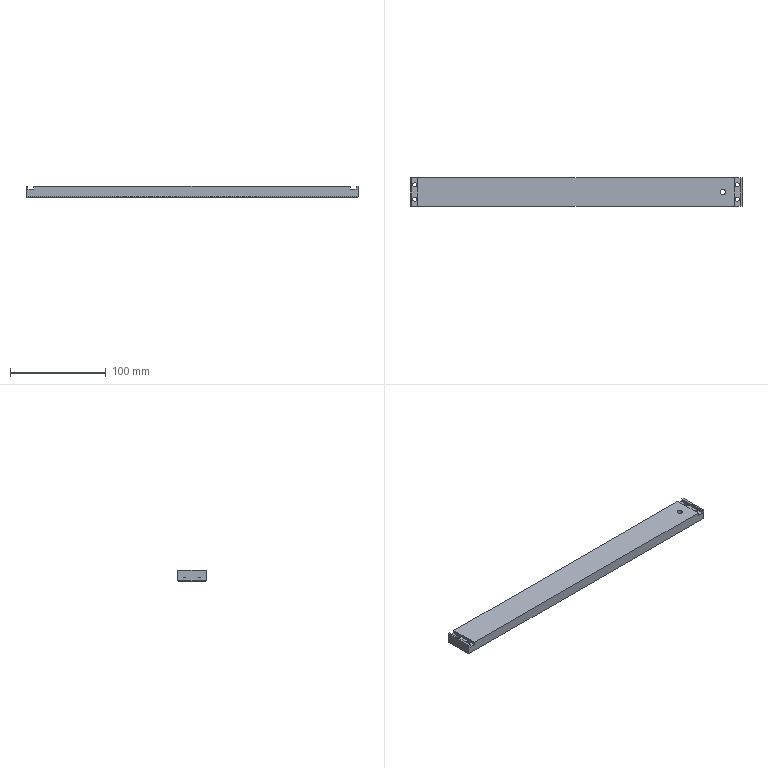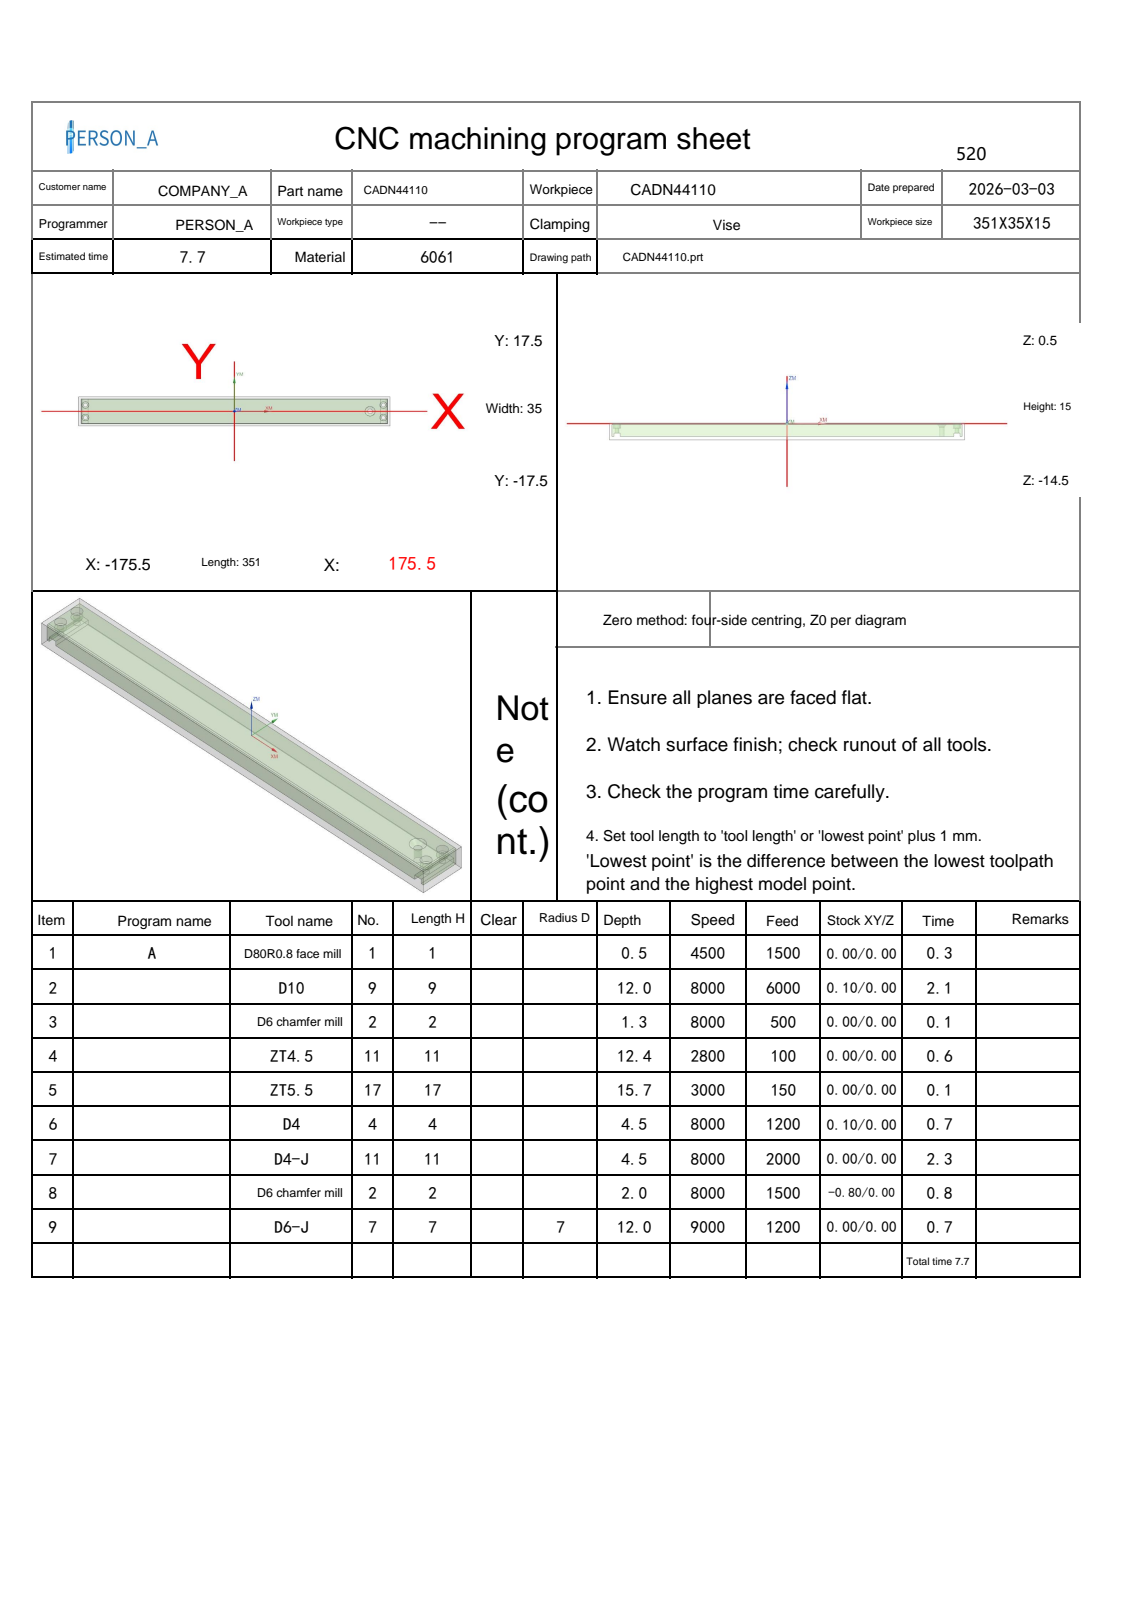NC program | NX | posted by the shop | part box 346 x 30 x 11.5 mm
Lines 1 to 336 of 28539:
%
O0001
(Machine time: 9.54 MIN)
(===Total Tool:7===)
(T1=D80R0.8 face mill D=80. R=0.8 D- H01 Z=0.    )
(T9=D10     D=10.  R=0.   D-  H09 Z=-11.5 )
(T2=D6 chamfer mill D=6. R=0. D- H02 Z=-1.5  )
(T11=ZT4.5  D=4.5  DR_a=118 D-  H11 Z=-11.85)
(T17=ZT5.5  D=5.5  DR_a=118 D-  H17 Z=-15.15)
(T4=D4      D=4.   R=0.   D-  H04 Z=-4.   )
(T7=D6-J    D=6.   R=0.   D7  H07 Z=-11.5 )
G80 G90 G17 G49 G40
G91 G28 Z0
M01
N1 T01 M06
(D80R0.8 face mill D=80. R=0.8 H=01 ce=0.00 di=0.00)
G00 G90 G54 X218. Y0.0 M03 S4500
G43 H01 Z30.
M08
Z2.
G01 Z0.0 F1500.
X213.
X-213.
X-218.
Z2.
G00 Z30.
G91 G28 Z0.0
M05
M09
G91 G28 Z0.0
M01
N2 T09 M06
(D10  D=10. R=0. H=09 ce=0.10 di=0.00)
G00 G90 G54 X0.0 Y20.1 M03 S8000
G43 H09 Z30.
M08
Z.5
G01 X173. Z.323 F6000.
G02 X178.1 Y15. Z.315 I0.0 J-5.1
G01 Y-15. Z.285
G02 X173. Y-20.1 Z.277 I-5.1 J0.0
G01 X-173. Z-.077
G02 X-178.1 Y-15. Z-.085 I0.0 J5.1
G01 Y15. Z-.115
G02 X-173. Y20.1 Z-.123 I5.1 J0.0
G01 X173. Z-.477
G02 X178.1 Y15. Z-.485 I0.0 J-5.1
G01 Y-15. Z-.515
G02 X173. Y-20.1 Z-.523 I-5.1 J0.0
G01 X-173. Z-.877
G02 X-178.1 Y-15. Z-.885 I0.0 J5.1
G01 Y15. Z-.915
G02 X-173. Y20.1 Z-.923 I5.1 J0.0
G01 X173. Z-1.277
G02 X178.1 Y15. Z-1.285 I0.0 J-5.1
G01 Y-15. Z-1.315
G02 X173. Y-20.1 Z-1.323 I-5.1 J0.0
G01 X-173. Z-1.677
G02 X-178.1 Y-15. Z-1.685 I0.0 J5.1
G01 Y15. Z-1.715
G02 X-173. Y20.1 Z-1.723 I5.1 J0.0
G01 X173. Z-2.077
G02 X178.1 Y15. Z-2.085 I0.0 J-5.1
G01 Y-15. Z-2.115
G02 X173. Y-20.1 Z-2.123 I-5.1 J0.0
G01 X-173. Z-2.477
G02 X-178.1 Y-15. Z-2.485 I0.0 J5.1
G01 Y15. Z-2.515
G02 X-173. Y20.1 Z-2.523 I5.1 J0.0
G01 X173. Z-2.877
G02 X178.1 Y15. Z-2.885 I0.0 J-5.1
G01 Y-15. Z-2.915
G02 X173. Y-20.1 Z-2.923 I-5.1 J0.0
G01 X-173. Z-3.277
G02 X-178.1 Y-15. Z-3.285 I0.0 J5.1
G01 Y15. Z-3.315
G02 X-173. Y20.1 Z-3.323 I5.1 J0.0
G01 X173. Z-3.677
G02 X178.1 Y15. Z-3.685 I0.0 J-5.1
G01 Y-15. Z-3.715
G02 X173. Y-20.1 Z-3.723 I-5.1 J0.0
G01 X-173. Z-4.077
G02 X-178.1 Y-15. Z-4.085 I0.0 J5.1
G01 Y15. Z-4.115
G02 X-173. Y20.1 Z-4.123 I5.1 J0.0
G01 X173. Z-4.477
G02 X178.1 Y15. Z-4.485 I0.0 J-5.1
G01 Y-15. Z-4.515
G02 X173. Y-20.1 Z-4.523 I-5.1 J0.0
G01 X-173. Z-4.877
G02 X-178.1 Y-15. Z-4.885 I0.0 J5.1
G01 Y15. Z-4.915
G02 X-173. Y20.1 Z-4.923 I5.1 J0.0
G01 X173. Z-5.277
G02 X178.1 Y15. Z-5.285 I0.0 J-5.1
G01 Y-15. Z-5.315
G02 X173. Y-20.1 Z-5.323 I-5.1 J0.0
G01 X-173. Z-5.677
G02 X-178.1 Y-15. Z-5.685 I0.0 J5.1
G01 Y15. Z-5.715
G02 X-173. Y20.1 Z-5.723 I5.1 J0.0
G01 X173. Z-6.077
G02 X178.1 Y15. Z-6.085 I0.0 J-5.1
G01 Y-15. Z-6.115
G02 X173. Y-20.1 Z-6.123 I-5.1 J0.0
G01 X-173. Z-6.477
G02 X-178.1 Y-15. Z-6.485 I0.0 J5.1
G01 Y15. Z-6.515
G02 X-173. Y20.1 Z-6.523 I5.1 J0.0
G01 X173. Z-6.877
G02 X178.1 Y15. Z-6.885 I0.0 J-5.1
G01 Y-15. Z-6.915
G02 X173. Y-20.1 Z-6.923 I-5.1 J0.0
G01 X-173. Z-7.277
G02 X-178.1 Y-15. Z-7.285 I0.0 J5.1
G01 Y15. Z-7.315
G02 X-173. Y20.1 Z-7.323 I5.1 J0.0
G01 X173. Z-7.677
G02 X178.1 Y15. Z-7.685 I0.0 J-5.1
G01 Y-15. Z-7.715
G02 X173. Y-20.1 Z-7.723 I-5.1 J0.0
G01 X-173. Z-8.077
G02 X-178.1 Y-15. Z-8.085 I0.0 J5.1
G01 Y15. Z-8.115
G02 X-173. Y20.1 Z-8.123 I5.1 J0.0
G01 X173. Z-8.477
G02 X178.1 Y15. Z-8.485 I0.0 J-5.1
G01 Y-15. Z-8.515
G02 X173. Y-20.1 Z-8.523 I-5.1 J0.0
G01 X-173. Z-8.877
G02 X-178.1 Y-15. Z-8.885 I0.0 J5.1
G01 Y15. Z-8.915
G02 X-173. Y20.1 Z-8.923 I5.1 J0.0
G01 X173. Z-9.277
G02 X178.1 Y15. Z-9.285 I0.0 J-5.1
G01 Y-15. Z-9.315
G02 X173. Y-20.1 Z-9.323 I-5.1 J0.0
G01 X-173. Z-9.677
G02 X-178.1 Y-15. Z-9.685 I0.0 J5.1
G01 Y15. Z-9.715
G02 X-173. Y20.1 Z-9.723 I5.1 J0.0
G01 X173. Z-10.077
G02 X178.1 Y15. Z-10.085 I0.0 J-5.1
G01 Y-15. Z-10.115
G02 X173. Y-20.1 Z-10.123 I-5.1 J0.0
G01 X-173. Z-10.477
G02 X-178.1 Y-15. Z-10.485 I0.0 J5.1
G01 Y15. Z-10.515
G02 X-173. Y20.1 Z-10.523 I5.1 J0.0
G01 X173. Z-10.877
G02 X178.1 Y15. Z-10.885 I0.0 J-5.1
G01 Y-15. Z-10.915
G02 X173. Y-20.1 Z-10.923 I-5.1 J0.0
G01 X-173. Z-11.277
G02 X-178.1 Y-15. Z-11.285 I0.0 J5.1
G01 Y15. Z-11.315
G02 X-173. Y20.1 Z-11.323 I5.1 J0.0
G01 X0.0 Z-11.5
X173.
G02 X178.1 Y15. I0.0 J-5.1
G01 Y-15.
G02 X173. Y-20.1 I-5.1 J0.0
G01 X-173.
G02 X-178.1 Y-15. I0.0 J5.1
G01 Y15.
G02 X-173. Y20.1 I5.1 J0.0
G01 X0.0
X.5
Z-10.5
G00 Z30.
G91 G28 Z0.0
M05
M09
G91 G28 Z0.0
M01
N3 T02 M06
(D6 chamfer mill D=6. R=0. H=02 ce=0.00 di=0.00)
G00 G90 G54 X168. Y7.5 M03 S8000
G43 H02 Z30.
M08
G98 G81 X168. Y7.5 Z-.8 R1. F500.
Y-7.5
X153. Y0.0
X-168. Y7.5
Y-7.5
G80
G00 Z30.
G91 G28 Z0.0
M05
M09
G91 G28 Z0.0
M01
N4 T11 M06
(ZT4.5 D=4.5 DR_a=118 H=11)
G00 G90 G54 X168. Y7.5 M03 S2800
G43 H11 Z30.
M08
G98 G83 X168. Y7.5 Z-11.852 R1. F100. Q2.
Y-7.5
X-168.
Y7.5
G80
G00 Z30.
G91 G28 Z0.0
M05
M09
G91 G28 Z0.0
M01
N5 T17 M06
(ZT5.5 D=5.5 DR_a=118 H=17)
G00 G90 G54 X153. Y0.0 M03 S3000
G43 H17 Z30.
M08
G98 G83 X153. Y0.0 Z-15.152 R1. F150. Q3.
G80
G00 Z30.
G91 G28 Z0.0
M05
M09
G91 G28 Z0.0
M01
N6 T04 M06
(D4  D=4. R=0. H=04 ce=0.10 di=0.00)
G00 G90 G54 X168. Y7.5 M03 S8000
G43 H04 Z30.
M08
Z.5
G03 X168.95 Y6.55 I.95 J0.0 F1200.
X169.9 Y7.5 I0.0 J.95
X169.9 Y7.5 Z.2 I-1.9 J0.0
X169.9 Y7.5 Z-.1 I-1.9 J0.0
X169.9 Y7.5 Z-.4 I-1.9 J0.0
X169.9 Y7.5 Z-.7 I-1.9 J0.0
X169.9 Y7.5 Z-1. I-1.9 J0.0
X169.9 Y7.5 Z-1.3 I-1.9 J0.0
X169.9 Y7.5 Z-1.6 I-1.9 J0.0
X169.9 Y7.5 Z-1.9 I-1.9 J0.0
X169.9 Y7.5 Z-2.2 I-1.9 J0.0
X169.9 Y7.5 Z-2.5 I-1.9 J0.0
X169.9 Y7.5 Z-2.8 I-1.9 J0.0
X169.9 Y7.5 Z-3.1 I-1.9 J0.0
X169.9 Y7.5 Z-3.4 I-1.9 J0.0
X169.9 Y7.5 Z-3.7 I-1.9 J0.0
X169.9 Y7.5 Z-4. I-1.9 J0.0
X168. Y9.4 I-1.9 J0.0
X166.1 Y7.5 I0.0 J-1.9
X168. Y5.6 I1.9 J0.0
X169.9 Y7.5 I0.0 J1.9
X168.95 Y8.45 I-.95 J0.0
X168. Y7.5 I0.0 J-.95
G00 Z30.
Y-7.5
Z.5
G03 X168.95 Y-8.45 I.95 J0.0
X169.9 Y-7.5 I0.0 J.95
X169.9 Y-7.5 Z.2 I-1.9 J0.0
X169.9 Y-7.5 Z-.1 I-1.9 J0.0
X169.9 Y-7.5 Z-.4 I-1.9 J0.0
X169.9 Y-7.5 Z-.7 I-1.9 J0.0
X169.9 Y-7.5 Z-1. I-1.9 J0.0
X169.9 Y-7.5 Z-1.3 I-1.9 J0.0
X169.9 Y-7.5 Z-1.6 I-1.9 J0.0
X169.9 Y-7.5 Z-1.9 I-1.9 J0.0
X169.9 Y-7.5 Z-2.2 I-1.9 J0.0
X169.9 Y-7.5 Z-2.5 I-1.9 J0.0
X169.9 Y-7.5 Z-2.8 I-1.9 J0.0
X169.9 Y-7.5 Z-3.1 I-1.9 J0.0
X169.9 Y-7.5 Z-3.4 I-1.9 J0.0
X169.9 Y-7.5 Z-3.7 I-1.9 J0.0
X169.9 Y-7.5 Z-4. I-1.9 J0.0
X168. Y-5.6 I-1.9 J0.0
X166.1 Y-7.5 I0.0 J-1.9
X168. Y-9.4 I1.9 J0.0
X169.9 Y-7.5 I0.0 J1.9
X168.95 Y-6.55 I-.95 J0.0
X168. Y-7.5 I0.0 J-.95
G00 Z30.
X-168.
Z.5
G03 X-167.05 Y-8.45 I.95 J0.0
X-166.1 Y-7.5 I0.0 J.95
X-166.1 Y-7.5 Z.2 I-1.9 J0.0
X-166.1 Y-7.5 Z-.1 I-1.9 J0.0
X-166.1 Y-7.5 Z-.4 I-1.9 J0.0
X-166.1 Y-7.5 Z-.7 I-1.9 J0.0
X-166.1 Y-7.5 Z-1. I-1.9 J0.0
X-166.1 Y-7.5 Z-1.3 I-1.9 J0.0
X-166.1 Y-7.5 Z-1.6 I-1.9 J0.0
X-166.1 Y-7.5 Z-1.9 I-1.9 J0.0
X-166.1 Y-7.5 Z-2.2 I-1.9 J0.0
X-166.1 Y-7.5 Z-2.5 I-1.9 J0.0
X-166.1 Y-7.5 Z-2.8 I-1.9 J0.0
X-166.1 Y-7.5 Z-3.1 I-1.9 J0.0
X-166.1 Y-7.5 Z-3.4 I-1.9 J0.0
X-166.1 Y-7.5 Z-3.7 I-1.9 J0.0
X-166.1 Y-7.5 Z-4. I-1.9 J0.0
X-168. Y-5.6 I-1.9 J0.0
X-169.9 Y-7.5 I0.0 J-1.9
X-168. Y-9.4 I1.9 J0.0
X-166.1 Y-7.5 I0.0 J1.9
X-167.05 Y-6.55 I-.95 J0.0
X-168. Y-7.5 I0.0 J-.95
G00 Z30.
Y7.5
Z.5
G03 X-167.05 Y6.55 I.95 J0.0
X-166.1 Y7.5 I0.0 J.95
X-166.1 Y7.5 Z.2 I-1.9 J0.0
X-166.1 Y7.5 Z-.1 I-1.9 J0.0
X-166.1 Y7.5 Z-.4 I-1.9 J0.0
X-166.1 Y7.5 Z-.7 I-1.9 J0.0
X-166.1 Y7.5 Z-1. I-1.9 J0.0
X-166.1 Y7.5 Z-1.3 I-1.9 J0.0
X-166.1 Y7.5 Z-1.6 I-1.9 J0.0
X-166.1 Y7.5 Z-1.9 I-1.9 J0.0
X-166.1 Y7.5 Z-2.2 I-1.9 J0.0
X-166.1 Y7.5 Z-2.5 I-1.9 J0.0
X-166.1 Y7.5 Z-2.8 I-1.9 J0.0
X-166.1 Y7.5 Z-3.1 I-1.9 J0.0
X-166.1 Y7.5 Z-3.4 I-1.9 J0.0
X-166.1 Y7.5 Z-3.7 I-1.9 J0.0
X-166.1 Y7.5 Z-4. I-1.9 J0.0
X-168. Y9.4 I-1.9 J0.0
X-169.9 Y7.5 I0.0 J-1.9
X-168. Y5.6 I1.9 J0.0
X-166.1 Y7.5 I0.0 J1.9
X-167.05 Y8.45 I-.95 J0.0
X-168. Y7.5 I0.0 J-.95
G00 Z30.
G91 G28 Z0.0
M05
M09
G91 G28 Z0.0
M01